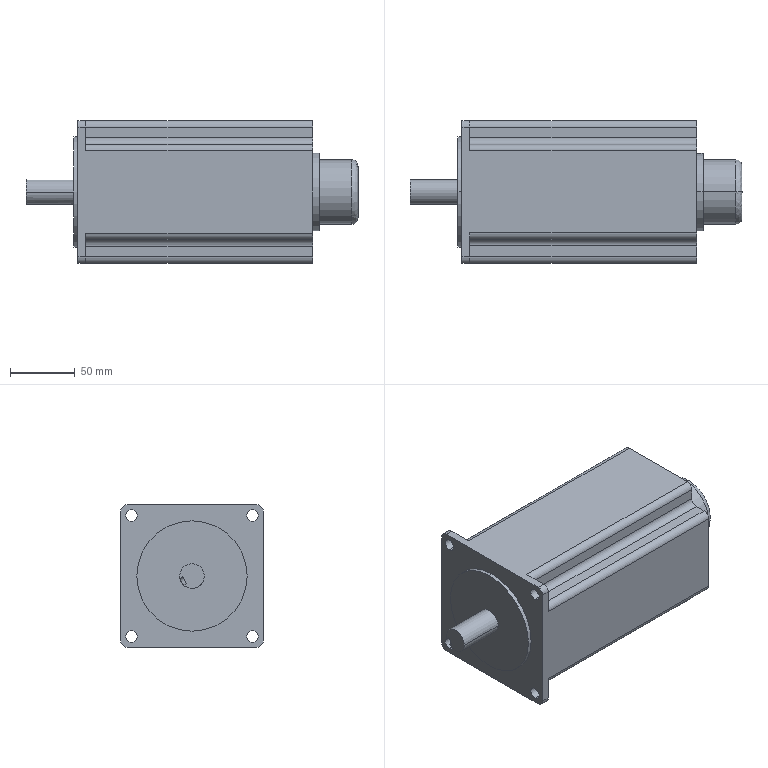Part | STEP file | BSHB311 Baishan Motor | 1 solid | 60 faces | box 256 x 110 x 110 mm | volume 2048364 mm3 | cylinder 33 | plane 25 | spline 2 | commonest cylinder face diameters 10 x16 9 x8 19 x2 50 x2 60 x2 85 x2